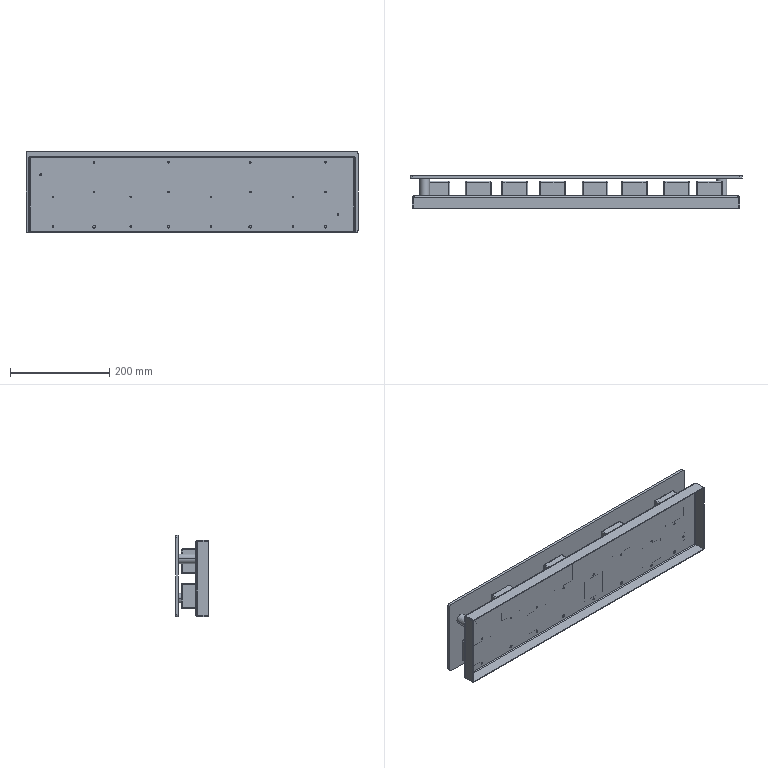Part | NX | 12 solids | 344 faces | box 670 x 66 x 164 mm | volume 1399817 mm3 | cylinder 144 | plane 96 | cone 72 | sphere 32 | commonest cylinder face diameters 4 x64 3.3 x52 5.5 x8 3.2 x4 6 x4 6.4 x4